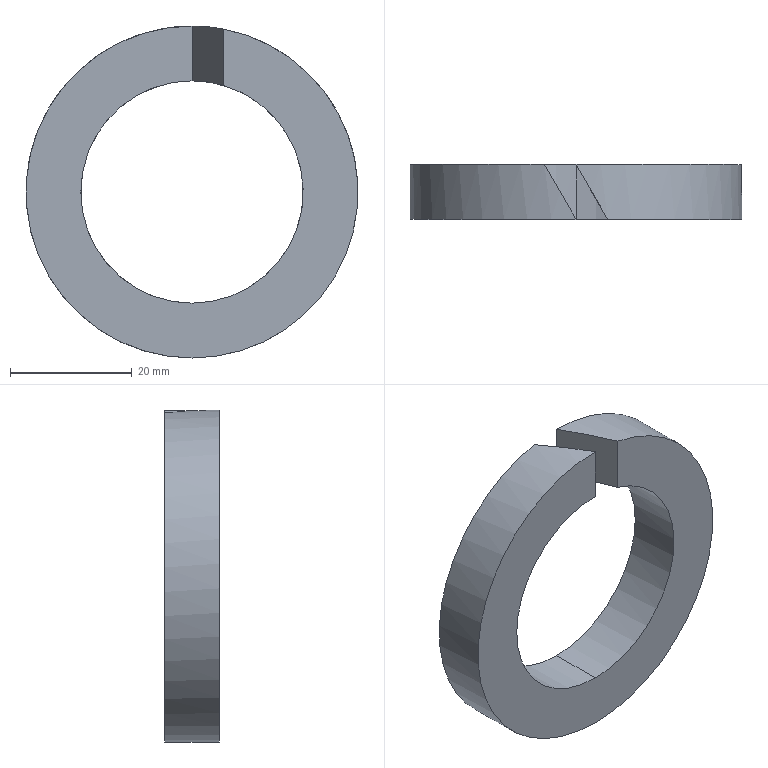Part | SolidWorks | features Extrusion 1, ICE 1 | 1 solid | 8 faces | box 54.5 x 9 x 54.5 mm | volume 11156 mm3 | cylinder 4 | plane 4 | commonest cylinder face diameters 36.5 x2 54.5 x2
STEP:
#1=CARTESIAN_POINT('',(0.,4.5,18.25));
#2=VERTEX_POINT('',#1);
#3=CARTESIAN_POINT('',(0.,4.5,-18.25));
#4=VERTEX_POINT('',#3);
#5=CARTESIAN_POINT('',(0.,4.5,0.));
#6=DIRECTION('',(0.,1.,0.));
#7=DIRECTION('',(0.,0.,1.));
#8=AXIS2_PLACEMENT_3D('',#5,#6,#7);
#9=CIRCLE('',#8,18.25);
#10=EDGE_CURVE('',#2,#4,#9,.T.);
#11=ORIENTED_EDGE('',*,*,#10,.T.);
#12=CARTESIAN_POINT('',(0.,-4.5,-18.25));
#13=VERTEX_POINT('',#12);
#14=CARTESIAN_POINT('',(0.,4.5,-18.25));
#15=DIRECTION('',(0.,-1.,0.));
#16=VECTOR('',#15,1000.);
#17=LINE('',#14,#16);
#18=EDGE_CURVE('',#4,#13,#17,.T.);
#19=ORIENTED_EDGE('',*,*,#18,.T.);
#20=CARTESIAN_POINT('',(5.196,-4.5,17.495));
#21=VERTEX_POINT('',#20);
#22=CARTESIAN_POINT('',(0.,-4.5,0.));
#23=DIRECTION('',(0.,1.,0.));
#24=DIRECTION('',(0.,0.,1.));
#25=AXIS2_PLACEMENT_3D('',#22,#23,#24);
#26=CIRCLE('',#25,18.25);
#27=EDGE_CURVE('',#21,#13,#26,.T.);
#28=ORIENTED_EDGE('',*,*,#27,.F.);
#29=CARTESIAN_POINT('',(5.196,-4.5,17.495));
#30=CARTESIAN_POINT('',(3.507,-1.574,17.996));
#31=CARTESIAN_POINT('',(1.762,1.447,18.25));
#32=CARTESIAN_POINT('',(0.,4.5,18.25));
#33=(BOUNDED_CURVE()B_SPLINE_CURVE(3,(#29,#30,#31,#32),.UNSPECIFIED.,.F.,.T.)B_SPLINE_CURVE_WITH_KNOTS((4,4),(1.282,1.571),.UNSPECIFIED.)CURVE()GEOMETRIC_REPRESENTATION_ITEM()RATIONAL_B_SPLINE_CURVE((1.,0.9931,0.9931,1.))REPRESENTATION_ITEM(''));
#34=EDGE_CURVE('',#21,#2,#33,.T.);
#35=ORIENTED_EDGE('',*,*,#34,.T.);
#36=EDGE_LOOP('',(#11,#19,#28,#35));
#37=FACE_OUTER_BOUND('',#36,.T.);
#38=CARTESIAN_POINT('',(0.,4.5,0.));
#39=DIRECTION('',(0.,-1.,0.));
#40=DIRECTION('',(0.,0.,-1.));
#41=AXIS2_PLACEMENT_3D('',#38,#39,#40);
#42=CYLINDRICAL_SURFACE('',#41,18.25);
#43=ADVANCED_FACE('',(#37),#42,.F.);
#44=CARTESIAN_POINT('',(0.,4.5,-27.25));
#45=VERTEX_POINT('',#44);
#46=CARTESIAN_POINT('',(-5.196,4.5,26.75));
#47=VERTEX_POINT('',#46);
#48=CARTESIAN_POINT('',(0.,4.5,0.));
#49=DIRECTION('',(0.,1.,0.));
#50=DIRECTION('',(0.,0.,1.));
#51=AXIS2_PLACEMENT_3D('',#48,#49,#50);
#52=CIRCLE('',#51,27.25);
#53=EDGE_CURVE('',#45,#47,#52,.T.);
#54=ORIENTED_EDGE('',*,*,#53,.F.);
#55=CARTESIAN_POINT('',(0.,-4.5,-27.25));
#56=VERTEX_POINT('',#55);
#57=CARTESIAN_POINT('',(0.,4.5,-27.25));
#58=DIRECTION('',(0.,-1.,0.));
#59=VECTOR('',#58,1000.);
#60=LINE('',#57,#59);
#61=EDGE_CURVE('',#45,#56,#60,.T.);
#62=ORIENTED_EDGE('',*,*,#61,.T.);
#63=CARTESIAN_POINT('',(0.,-4.5,27.25));
#64=VERTEX_POINT('',#63);
#65=CARTESIAN_POINT('',(0.,-4.5,0.));
#66=DIRECTION('',(0.,1.,0.));
#67=DIRECTION('',(0.,0.,1.));
#68=AXIS2_PLACEMENT_3D('',#65,#66,#67);
#69=CIRCLE('',#68,27.25);
#70=EDGE_CURVE('',#56,#64,#69,.T.);
#71=ORIENTED_EDGE('',*,*,#70,.T.);
#72=CARTESIAN_POINT('',(-5.196,4.5,26.75));
#73=CARTESIAN_POINT('',(-3.483,1.532,27.083));
#74=CARTESIAN_POINT('',(-1.745,-1.477,27.25));
#75=CARTESIAN_POINT('',(0.,-4.5,27.25));
#76=(BOUNDED_CURVE()B_SPLINE_CURVE(3,(#72,#73,#74,#75),.UNSPECIFIED.,.F.,.T.)B_SPLINE_CURVE_WITH_KNOTS((4,4),(4.521,4.712),.UNSPECIFIED.)CURVE()GEOMETRIC_REPRESENTATION_ITEM()RATIONAL_B_SPLINE_CURVE((1.,0.9969,0.9969,1.))REPRESENTATION_ITEM(''));
#77=EDGE_CURVE('',#47,#64,#76,.T.);
#78=ORIENTED_EDGE('',*,*,#77,.F.);
#79=EDGE_LOOP('',(#54,#62,#71,#78));
#80=FACE_OUTER_BOUND('',#79,.T.);
#81=CARTESIAN_POINT('',(0.,4.5,0.));
#82=DIRECTION('',(0.,-1.,0.));
#83=DIRECTION('',(0.,0.,-1.));
#84=AXIS2_PLACEMENT_3D('',#81,#82,#83);
#85=CYLINDRICAL_SURFACE('',#84,27.25);
#86=ADVANCED_FACE('',(#80),#85,.T.);
#87=ORIENTED_EDGE('',*,*,#10,.F.);
#88=CARTESIAN_POINT('',(0.,4.5,27.25));
#89=VERTEX_POINT('',#88);
#90=CARTESIAN_POINT('',(0.,4.5,27.25));
#91=DIRECTION('',(0.,0.,-1.));
#92=VECTOR('',#91,1000.);
#93=LINE('',#90,#92);
#94=EDGE_CURVE('',#89,#2,#93,.T.);
#95=ORIENTED_EDGE('',*,*,#94,.F.);
#96=CARTESIAN_POINT('',(0.,4.5,0.));
#97=DIRECTION('',(0.,1.,0.));
#98=DIRECTION('',(0.,0.,1.));
#99=AXIS2_PLACEMENT_3D('',#96,#97,#98);
#100=CIRCLE('',#99,27.25);
#101=EDGE_CURVE('',#89,#45,#100,.T.);
#102=ORIENTED_EDGE('',*,*,#101,.T.);
#103=ORIENTED_EDGE('',*,*,#53,.T.);
#104=CARTESIAN_POINT('',(-5.196,4.5,17.495));
#105=VERTEX_POINT('',#104);
#106=CARTESIAN_POINT('',(-5.196,4.5,27.25));
#107=DIRECTION('',(0.,0.,-1.));
#108=VECTOR('',#107,1000.);
#109=LINE('',#106,#108);
#110=EDGE_CURVE('',#47,#105,#109,.T.);
#111=ORIENTED_EDGE('',*,*,#110,.T.);
#112=CARTESIAN_POINT('',(0.,4.5,0.));
#113=DIRECTION('',(0.,1.,0.));
#114=DIRECTION('',(0.,0.,1.));
#115=AXIS2_PLACEMENT_3D('',#112,#113,#114);
#116=CIRCLE('',#115,18.25);
#117=EDGE_CURVE('',#4,#105,#116,.T.);
#118=ORIENTED_EDGE('',*,*,#117,.F.);
#119=EDGE_LOOP('',(#87,#95,#102,#103,#111,#118));
#120=FACE_OUTER_BOUND('',#119,.T.);
#121=CARTESIAN_POINT('',(0.,4.5,0.));
#122=DIRECTION('',(0.,1.,0.));
#123=DIRECTION('',(0.,0.,1.));
#124=AXIS2_PLACEMENT_3D('',#121,#122,#123);
#125=PLANE('',#124);
#126=ADVANCED_FACE('',(#120),#125,.T.);
#127=CARTESIAN_POINT('',(5.196,-4.5,26.75));
#128=VERTEX_POINT('',#127);
#129=CARTESIAN_POINT('',(5.196,-4.5,27.25));
#130=DIRECTION('',(0.,0.,-1.));
#131=VECTOR('',#130,1000.);
#132=LINE('',#129,#131);
#133=EDGE_CURVE('',#128,#21,#132,.T.);
#134=ORIENTED_EDGE('',*,*,#133,.T.);
#135=ORIENTED_EDGE('',*,*,#27,.T.);
#136=CARTESIAN_POINT('',(0.,-4.5,18.25));
#137=VERTEX_POINT('',#136);
#138=CARTESIAN_POINT('',(0.,-4.5,0.));
#139=DIRECTION('',(0.,1.,0.));
#140=DIRECTION('',(0.,0.,1.));
#141=AXIS2_PLACEMENT_3D('',#138,#139,#140);
#142=CIRCLE('',#141,18.25);
#143=EDGE_CURVE('',#13,#137,#142,.T.);
#144=ORIENTED_EDGE('',*,*,#143,.T.);
#145=CARTESIAN_POINT('',(0.,-4.5,27.25));
#146=DIRECTION('',(0.,0.,-1.));
#147=VECTOR('',#146,1000.);
#148=LINE('',#145,#147);
#149=EDGE_CURVE('',#64,#137,#148,.T.);
#150=ORIENTED_EDGE('',*,*,#149,.F.);
#151=ORIENTED_EDGE('',*,*,#70,.F.);
#152=CARTESIAN_POINT('',(0.,-4.5,0.));
#153=DIRECTION('',(0.,1.,0.));
#154=DIRECTION('',(0.,0.,1.));
#155=AXIS2_PLACEMENT_3D('',#152,#153,#154);
#156=CIRCLE('',#155,27.25);
#157=EDGE_CURVE('',#128,#56,#156,.T.);
#158=ORIENTED_EDGE('',*,*,#157,.F.);
#159=EDGE_LOOP('',(#134,#135,#144,#150,#151,#158));
#160=FACE_OUTER_BOUND('',#159,.T.);
#161=CARTESIAN_POINT('',(0.,-4.5,0.));
#162=DIRECTION('',(0.,1.,0.));
#163=DIRECTION('',(0.,0.,1.));
#164=AXIS2_PLACEMENT_3D('',#161,#162,#163);
#165=PLANE('',#164);
#166=ADVANCED_FACE('',(#160),#165,.F.);
#167=ORIENTED_EDGE('',*,*,#61,.F.);
#168=ORIENTED_EDGE('',*,*,#101,.F.);
#169=CARTESIAN_POINT('',(5.196,-4.5,26.75));
#170=CARTESIAN_POINT('',(3.483,-1.532,27.083));
#171=CARTESIAN_POINT('',(1.745,1.477,27.25));
#172=CARTESIAN_POINT('',(0.,4.5,27.25));
#173=(BOUNDED_CURVE()B_SPLINE_CURVE(3,(#169,#170,#171,#172),.UNSPECIFIED.,.F.,.F.)B_SPLINE_CURVE_WITH_KNOTS((4,4),(1.379,1.571),.UNSPECIFIED.)CURVE()GEOMETRIC_REPRESENTATION_ITEM()RATIONAL_B_SPLINE_CURVE((1.,0.9969,0.9969,1.))REPRESENTATION_ITEM(''));
#174=EDGE_CURVE('',#128,#89,#173,.T.);
#175=ORIENTED_EDGE('',*,*,#174,.F.);
#176=ORIENTED_EDGE('',*,*,#157,.T.);
#177=EDGE_LOOP('',(#167,#168,#175,#176));
#178=FACE_OUTER_BOUND('',#177,.T.);
#179=CARTESIAN_POINT('',(0.,4.5,0.));
#180=DIRECTION('',(0.,-1.,0.));
#181=DIRECTION('',(0.,0.,-1.));
#182=AXIS2_PLACEMENT_3D('',#179,#180,#181);
#183=CYLINDRICAL_SURFACE('',#182,27.25);
#184=ADVANCED_FACE('',(#178),#183,.T.);
#185=ORIENTED_EDGE('',*,*,#18,.F.);
#186=ORIENTED_EDGE('',*,*,#117,.T.);
#187=CARTESIAN_POINT('',(-5.196,4.5,17.495));
#188=CARTESIAN_POINT('',(-3.507,1.574,17.996));
#189=CARTESIAN_POINT('',(-1.762,-1.447,18.25));
#190=CARTESIAN_POINT('',(0.,-4.5,18.25));
#191=(BOUNDED_CURVE()B_SPLINE_CURVE(3,(#187,#188,#189,#190),.UNSPECIFIED.,.F.,.F.)B_SPLINE_CURVE_WITH_KNOTS((4,4),(4.424,4.712),.UNSPECIFIED.)CURVE()GEOMETRIC_REPRESENTATION_ITEM()RATIONAL_B_SPLINE_CURVE((1.,0.9931,0.9931,1.))REPRESENTATION_ITEM(''));
#192=EDGE_CURVE('',#105,#137,#191,.T.);
#193=ORIENTED_EDGE('',*,*,#192,.T.);
#194=ORIENTED_EDGE('',*,*,#143,.F.);
#195=EDGE_LOOP('',(#185,#186,#193,#194));
#196=FACE_OUTER_BOUND('',#195,.T.);
#197=CARTESIAN_POINT('',(0.,4.5,0.));
#198=DIRECTION('',(0.,-1.,0.));
#199=DIRECTION('',(0.,0.,-1.));
#200=AXIS2_PLACEMENT_3D('',#197,#198,#199);
#201=CYLINDRICAL_SURFACE('',#200,18.25);
#202=ADVANCED_FACE('',(#196),#201,.F.);
#203=ORIENTED_EDGE('',*,*,#77,.T.);
#204=ORIENTED_EDGE('',*,*,#149,.T.);
#205=ORIENTED_EDGE('',*,*,#192,.F.);
#206=ORIENTED_EDGE('',*,*,#110,.F.);
#207=EDGE_LOOP('',(#203,#204,#205,#206));
#208=FACE_OUTER_BOUND('',#207,.T.);
#209=CARTESIAN_POINT('',(-5.196,4.5,27.25));
#210=DIRECTION('',(0.866,0.5,0.));
#211=DIRECTION('',(-0.5,0.866,0.));
#212=AXIS2_PLACEMENT_3D('',#209,#210,#211);
#213=PLANE('',#212);
#214=ADVANCED_FACE('',(#208),#213,.T.);
#215=ORIENTED_EDGE('',*,*,#174,.T.);
#216=ORIENTED_EDGE('',*,*,#94,.T.);
#217=ORIENTED_EDGE('',*,*,#34,.F.);
#218=ORIENTED_EDGE('',*,*,#133,.F.);
#219=EDGE_LOOP('',(#215,#216,#217,#218));
#220=FACE_OUTER_BOUND('',#219,.T.);
#221=CARTESIAN_POINT('',(0.,4.5,27.25));
#222=DIRECTION('',(-0.866,-0.5,0.));
#223=DIRECTION('',(0.5,-0.866,0.));
#224=AXIS2_PLACEMENT_3D('',#221,#222,#223);
#225=PLANE('',#224);
#226=ADVANCED_FACE('',(#220),#225,.T.);
#227=CLOSED_SHELL('',(#43,#86,#126,#166,#184,#202,#214,#226));
#228=MANIFOLD_SOLID_BREP('',#227);
#229=CARTESIAN_POINT('',(0.,0.,0.));
#230=DIRECTION('',(0.,0.,1.));
#231=DIRECTION('',(1.,0.,0.));
#232=AXIS2_PLACEMENT_3D('',#229,#230,#231);
#233=(LENGTH_UNIT()NAMED_UNIT(*)SI_UNIT(.MILLI.,.METRE.));
#234=UNCERTAINTY_MEASURE_WITH_UNIT(LENGTH_MEASURE(0.00001),#233,'','');
#235=(NAMED_UNIT(*)PLANE_ANGLE_UNIT()SI_UNIT($,.RADIAN.));
#236=(NAMED_UNIT(*)SI_UNIT($,.STERADIAN.)SOLID_ANGLE_UNIT());
#237=(GEOMETRIC_REPRESENTATION_CONTEXT(3)GLOBAL_UNCERTAINTY_ASSIGNED_CONTEXT((#234))GLOBAL_UNIT_ASSIGNED_CONTEXT((#233,#235,#236))REPRESENTATION_CONTEXT('',''));
#238=ADVANCED_BREP_SHAPE_REPRESENTATION('',(#228,#232),#237);